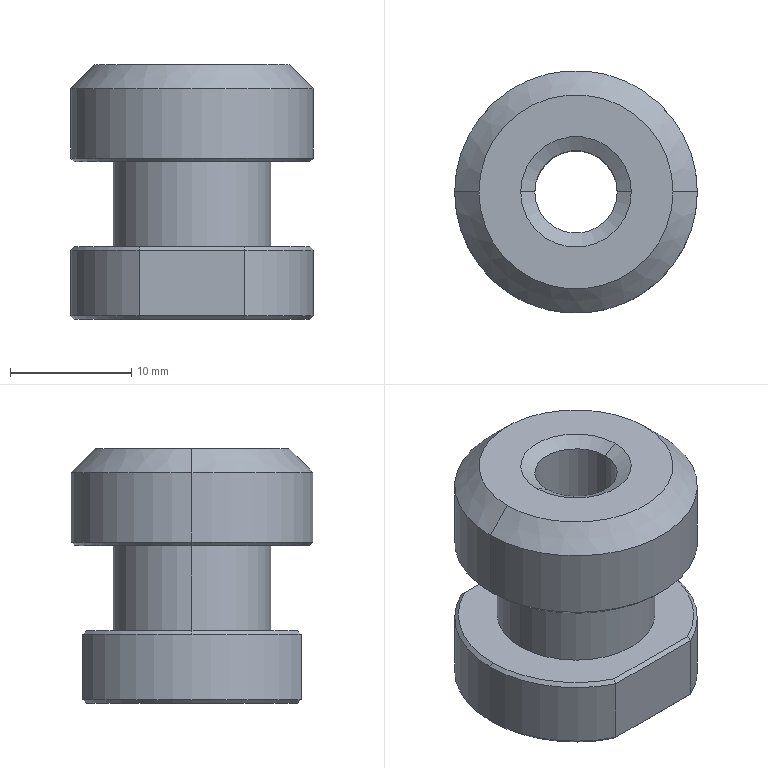Part | NX | 1 solid | 31 faces | box 20 x 20 x 21 mm | volume 4359 mm3 | cone 12 | plane 10 | cylinder 9 | commonest cylinder face diameters 20 x5 6.8 x2 13 x2
STEP:
#1=CARTESIAN_POINT('',(-93.533,-7.21,-2.7));
#2=VERTEX_POINT('',#1);
#3=CARTESIAN_POINT('',(-93.533,-7.21,2.7));
#4=VERTEX_POINT('',#3);
#5=CARTESIAN_POINT('',(-93.533,-7.21,-1.));
#6=DIRECTION('',(0.,0.,1.));
#7=VECTOR('',#6,1000.);
#8=LINE('',#5,#7);
#9=EDGE_CURVE('',#2,#4,#8,.T.);
#10=ORIENTED_EDGE('',*,*,#9,.F.);
#11=CARTESIAN_POINT('',(-99.174,1.79,-2.7));
#12=VERTEX_POINT('',#11);
#13=CARTESIAN_POINT('',(-103.533,-7.21,-2.7));
#14=DIRECTION('',(0.,0.,1.));
#15=DIRECTION('',(1.,0.,0.));
#16=AXIS2_PLACEMENT_3D('',#13,#14,#15);
#17=CIRCLE('',#16,10.);
#18=EDGE_CURVE('',#2,#12,#17,.T.);
#19=ORIENTED_EDGE('',*,*,#18,.T.);
#20=CARTESIAN_POINT('',(-99.174,1.79,2.7));
#21=VERTEX_POINT('',#20);
#22=CARTESIAN_POINT('',(-99.174,1.79,-1.));
#23=DIRECTION('',(0.,0.,1.));
#24=VECTOR('',#23,1000.);
#25=LINE('',#22,#24);
#26=EDGE_CURVE('',#12,#21,#25,.T.);
#27=ORIENTED_EDGE('',*,*,#26,.T.);
#28=CARTESIAN_POINT('',(-103.533,-7.21,2.7));
#29=DIRECTION('',(0.,0.,-1.));
#30=DIRECTION('',(-1.,0.,0.));
#31=AXIS2_PLACEMENT_3D('',#28,#29,#30);
#32=CIRCLE('',#31,10.);
#33=EDGE_CURVE('',#21,#4,#32,.T.);
#34=ORIENTED_EDGE('',*,*,#33,.T.);
#35=EDGE_LOOP('',(#10,#19,#27,#34));
#36=FACE_BOUND('',#35,.T.);
#37=CARTESIAN_POINT('',(-103.533,-7.21,-1.));
#38=DIRECTION('',(0.,0.,1.));
#39=DIRECTION('',(1.,0.,0.));
#40=AXIS2_PLACEMENT_3D('',#37,#38,#39);
#41=CYLINDRICAL_SURFACE('',#40,10.);
#42=ADVANCED_FACE('',(#36),#41,.T.);
#43=CARTESIAN_POINT('',(-107.892,1.79,-2.7));
#44=VERTEX_POINT('',#43);
#45=CARTESIAN_POINT('',(-107.892,1.79,2.7));
#46=VERTEX_POINT('',#45);
#47=CARTESIAN_POINT('',(-107.892,1.79,-1.));
#48=DIRECTION('',(0.,0.,1.));
#49=VECTOR('',#48,1000.);
#50=LINE('',#47,#49);
#51=EDGE_CURVE('',#44,#46,#50,.T.);
#52=ORIENTED_EDGE('',*,*,#51,.F.);
#53=CARTESIAN_POINT('',(-107.892,-16.21,-2.7));
#54=VERTEX_POINT('',#53);
#55=CARTESIAN_POINT('',(-103.533,-7.21,-2.7));
#56=DIRECTION('',(0.,0.,1.));
#57=DIRECTION('',(1.,0.,0.));
#58=AXIS2_PLACEMENT_3D('',#55,#56,#57);
#59=CIRCLE('',#58,10.);
#60=EDGE_CURVE('',#44,#54,#59,.T.);
#61=ORIENTED_EDGE('',*,*,#60,.T.);
#62=CARTESIAN_POINT('',(-107.892,-16.21,2.7));
#63=VERTEX_POINT('',#62);
#64=CARTESIAN_POINT('',(-107.892,-16.21,-1.));
#65=DIRECTION('',(0.,0.,1.));
#66=VECTOR('',#65,1000.);
#67=LINE('',#64,#66);
#68=EDGE_CURVE('',#54,#63,#67,.T.);
#69=ORIENTED_EDGE('',*,*,#68,.T.);
#70=CARTESIAN_POINT('',(-113.533,-7.21,2.7));
#71=VERTEX_POINT('',#70);
#72=CARTESIAN_POINT('',(-103.533,-7.21,2.7));
#73=DIRECTION('',(0.,0.,-1.));
#74=DIRECTION('',(-1.,0.,0.));
#75=AXIS2_PLACEMENT_3D('',#72,#73,#74);
#76=CIRCLE('',#75,10.);
#77=EDGE_CURVE('',#63,#71,#76,.T.);
#78=ORIENTED_EDGE('',*,*,#77,.T.);
#79=CARTESIAN_POINT('',(-103.533,-7.21,2.7));
#80=DIRECTION('',(0.,0.,-1.));
#81=DIRECTION('',(-1.,0.,0.));
#82=AXIS2_PLACEMENT_3D('',#79,#80,#81);
#83=CIRCLE('',#82,10.);
#84=EDGE_CURVE('',#71,#46,#83,.T.);
#85=ORIENTED_EDGE('',*,*,#84,.T.);
#86=EDGE_LOOP('',(#52,#61,#69,#78,#85));
#87=FACE_BOUND('',#86,.T.);
#88=CARTESIAN_POINT('',(-103.533,-7.21,-1.));
#89=DIRECTION('',(0.,0.,1.));
#90=DIRECTION('',(1.,0.,0.));
#91=AXIS2_PLACEMENT_3D('',#88,#89,#90);
#92=CYLINDRICAL_SURFACE('',#91,10.);
#93=ADVANCED_FACE('',(#87),#92,.T.);
#94=CARTESIAN_POINT('',(-99.174,-16.21,-2.7));
#95=VERTEX_POINT('',#94);
#96=CARTESIAN_POINT('',(-104.112,-16.21,-2.7));
#97=DIRECTION('',(-1.,0.,0.));
#98=VECTOR('',#97,1000.);
#99=LINE('',#96,#98);
#100=EDGE_CURVE('',#95,#54,#99,.T.);
#101=ORIENTED_EDGE('',*,*,#100,.F.);
#102=CARTESIAN_POINT('',(-99.174,-16.21,2.7));
#103=VERTEX_POINT('',#102);
#104=CARTESIAN_POINT('',(-99.174,-16.21,-1.));
#105=DIRECTION('',(0.,0.,1.));
#106=VECTOR('',#105,1000.);
#107=LINE('',#104,#106);
#108=EDGE_CURVE('',#95,#103,#107,.T.);
#109=ORIENTED_EDGE('',*,*,#108,.T.);
#110=CARTESIAN_POINT('',(-104.112,-16.21,2.7));
#111=DIRECTION('',(1.,0.,0.));
#112=VECTOR('',#111,1000.);
#113=LINE('',#110,#112);
#114=EDGE_CURVE('',#63,#103,#113,.T.);
#115=ORIENTED_EDGE('',*,*,#114,.F.);
#116=ORIENTED_EDGE('',*,*,#68,.F.);
#117=EDGE_LOOP('',(#101,#109,#115,#116));
#118=FACE_BOUND('',#117,.T.);
#119=CARTESIAN_POINT('',(-99.791,-16.21,-1.));
#120=DIRECTION('',(0.,-1.,0.));
#121=DIRECTION('',(0.,0.,-1.));
#122=AXIS2_PLACEMENT_3D('',#119,#120,#121);
#123=PLANE('',#122);
#124=ADVANCED_FACE('',(#118),#123,.T.);
#125=CARTESIAN_POINT('',(-99.243,-15.91,-3.));
#126=VERTEX_POINT('',#125);
#127=CARTESIAN_POINT('',(-107.822,-15.91,-3.));
#128=VERTEX_POINT('',#127);
#129=CARTESIAN_POINT('',(0.,-15.91,-3.));
#130=DIRECTION('',(-1.,0.,0.));
#131=VECTOR('',#130,1000.);
#132=LINE('',#129,#131);
#133=EDGE_CURVE('',#126,#128,#132,.T.);
#134=ORIENTED_EDGE('',*,*,#133,.F.);
#135=CARTESIAN_POINT('',(-99.174,-16.21,-2.7));
#136=CARTESIAN_POINT('',(-99.179,-16.185,-2.725));
#137=CARTESIAN_POINT('',(-99.185,-16.16,-2.75));
#138=CARTESIAN_POINT('',(-99.191,-16.135,-2.775));
#139=CARTESIAN_POINT('',(-99.197,-16.11,-2.8));
#140=CARTESIAN_POINT('',(-99.203,-16.085,-2.825));
#141=CARTESIAN_POINT('',(-99.208,-16.06,-2.85));
#142=CARTESIAN_POINT('',(-99.214,-16.035,-2.875));
#143=CARTESIAN_POINT('',(-99.22,-16.01,-2.9));
#144=CARTESIAN_POINT('',(-99.226,-15.985,-2.925));
#145=CARTESIAN_POINT('',(-99.231,-15.96,-2.95));
#146=CARTESIAN_POINT('',(-99.237,-15.935,-2.975));
#147=CARTESIAN_POINT('',(-99.243,-15.91,-3.));
#148=B_SPLINE_CURVE_WITH_KNOTS('',3,(#135,#136,#137,#138,#139,#140,#141,#142,#143,#144,#145,#146,#147),.UNSPECIFIED.,.F.,.F.,(4,3,3,3,4),(0.,0.1075,0.2149,0.3224,0.4299),.UNSPECIFIED.);
#149=EDGE_CURVE('',#95,#126,#148,.T.);
#150=ORIENTED_EDGE('',*,*,#149,.F.);
#151=ORIENTED_EDGE('',*,*,#100,.T.);
#152=CARTESIAN_POINT('',(-107.822,-15.91,-3.));
#153=CARTESIAN_POINT('',(-107.828,-15.935,-2.975));
#154=CARTESIAN_POINT('',(-107.834,-15.96,-2.95));
#155=CARTESIAN_POINT('',(-107.84,-15.985,-2.925));
#156=CARTESIAN_POINT('',(-107.845,-16.01,-2.9));
#157=CARTESIAN_POINT('',(-107.851,-16.035,-2.875));
#158=CARTESIAN_POINT('',(-107.857,-16.06,-2.85));
#159=CARTESIAN_POINT('',(-107.863,-16.085,-2.825));
#160=CARTESIAN_POINT('',(-107.869,-16.11,-2.8));
#161=CARTESIAN_POINT('',(-107.874,-16.135,-2.775));
#162=CARTESIAN_POINT('',(-107.88,-16.16,-2.75));
#163=CARTESIAN_POINT('',(-107.886,-16.185,-2.725));
#164=CARTESIAN_POINT('',(-107.892,-16.21,-2.7));
#165=B_SPLINE_CURVE_WITH_KNOTS('',3,(#152,#153,#154,#155,#156,#157,#158,#159,#160,#161,#162,#163,#164),.UNSPECIFIED.,.F.,.F.,(4,3,3,3,4),(0.,0.1075,0.2149,0.3224,0.4299),.UNSPECIFIED.);
#166=EDGE_CURVE('',#128,#54,#165,.T.);
#167=ORIENTED_EDGE('',*,*,#166,.F.);
#168=EDGE_LOOP('',(#134,#150,#151,#167));
#169=FACE_BOUND('',#168,.T.);
#170=CARTESIAN_POINT('',(-103.533,-16.06,-2.85));
#171=DIRECTION('',(0.,-0.7071,-0.7071));
#172=DIRECTION('',(0.,-0.7071,0.7071));
#173=AXIS2_PLACEMENT_3D('',#170,#171,#172);
#174=PLANE('',#173);
#175=ADVANCED_FACE('',(#169),#174,.T.);
#176=CARTESIAN_POINT('',(-107.822,1.49,-3.));
#177=VERTEX_POINT('',#176);
#178=CARTESIAN_POINT('',(-99.243,1.49,-3.));
#179=VERTEX_POINT('',#178);
#180=CARTESIAN_POINT('',(0.,1.49,-3.));
#181=DIRECTION('',(1.,0.,0.));
#182=VECTOR('',#181,1000.);
#183=LINE('',#180,#182);
#184=EDGE_CURVE('',#177,#179,#183,.T.);
#185=ORIENTED_EDGE('',*,*,#184,.F.);
#186=CARTESIAN_POINT('',(-107.892,1.79,-2.7));
#187=CARTESIAN_POINT('',(-107.886,1.765,-2.725));
#188=CARTESIAN_POINT('',(-107.88,1.74,-2.75));
#189=CARTESIAN_POINT('',(-107.874,1.715,-2.775));
#190=CARTESIAN_POINT('',(-107.869,1.69,-2.8));
#191=CARTESIAN_POINT('',(-107.863,1.665,-2.825));
#192=CARTESIAN_POINT('',(-107.857,1.64,-2.85));
#193=CARTESIAN_POINT('',(-107.851,1.615,-2.875));
#194=CARTESIAN_POINT('',(-107.845,1.59,-2.9));
#195=CARTESIAN_POINT('',(-107.84,1.565,-2.925));
#196=CARTESIAN_POINT('',(-107.834,1.54,-2.95));
#197=CARTESIAN_POINT('',(-107.828,1.515,-2.975));
#198=CARTESIAN_POINT('',(-107.822,1.49,-3.));
#199=B_SPLINE_CURVE_WITH_KNOTS('',3,(#186,#187,#188,#189,#190,#191,#192,#193,#194,#195,#196,#197,#198),.UNSPECIFIED.,.F.,.F.,(4,3,3,3,4),(0.,0.1075,0.2149,0.3224,0.4299),.UNSPECIFIED.);
#200=EDGE_CURVE('',#44,#177,#199,.T.);
#201=ORIENTED_EDGE('',*,*,#200,.F.);
#202=CARTESIAN_POINT('',(-104.112,1.79,-2.7));
#203=DIRECTION('',(1.,0.,0.));
#204=VECTOR('',#203,1000.);
#205=LINE('',#202,#204);
#206=EDGE_CURVE('',#44,#12,#205,.T.);
#207=ORIENTED_EDGE('',*,*,#206,.T.);
#208=CARTESIAN_POINT('',(-99.243,1.49,-3.));
#209=CARTESIAN_POINT('',(-99.237,1.515,-2.975));
#210=CARTESIAN_POINT('',(-99.231,1.54,-2.95));
#211=CARTESIAN_POINT('',(-99.226,1.565,-2.925));
#212=CARTESIAN_POINT('',(-99.22,1.59,-2.9));
#213=CARTESIAN_POINT('',(-99.214,1.615,-2.875));
#214=CARTESIAN_POINT('',(-99.208,1.64,-2.85));
#215=CARTESIAN_POINT('',(-99.203,1.665,-2.825));
#216=CARTESIAN_POINT('',(-99.197,1.69,-2.8));
#217=CARTESIAN_POINT('',(-99.191,1.715,-2.775));
#218=CARTESIAN_POINT('',(-99.185,1.74,-2.75));
#219=CARTESIAN_POINT('',(-99.179,1.765,-2.725));
#220=CARTESIAN_POINT('',(-99.174,1.79,-2.7));
#221=B_SPLINE_CURVE_WITH_KNOTS('',3,(#208,#209,#210,#211,#212,#213,#214,#215,#216,#217,#218,#219,#220),.UNSPECIFIED.,.F.,.F.,(4,3,3,3,4),(0.,0.1075,0.2149,0.3224,0.4299),.UNSPECIFIED.);
#222=EDGE_CURVE('',#179,#12,#221,.T.);
#223=ORIENTED_EDGE('',*,*,#222,.F.);
#224=EDGE_LOOP('',(#185,#201,#207,#223));
#225=FACE_BOUND('',#224,.T.);
#226=CARTESIAN_POINT('',(-103.533,1.64,-2.85));
#227=DIRECTION('',(0.,0.7071,-0.7071));
#228=DIRECTION('',(-1.,0.,0.));
#229=AXIS2_PLACEMENT_3D('',#226,#227,#228);
#230=PLANE('',#229);
#231=ADVANCED_FACE('',(#225),#230,.T.);
#232=CARTESIAN_POINT('',(-113.233,-7.21,10.));
#233=VERTEX_POINT('',#232);
#234=CARTESIAN_POINT('',(-93.833,-7.21,10.));
#235=VERTEX_POINT('',#234);
#236=CARTESIAN_POINT('',(-103.533,-7.21,10.));
#237=DIRECTION('',(0.,0.,1.));
#238=DIRECTION('',(1.,0.,0.));
#239=AXIS2_PLACEMENT_3D('',#236,#237,#238);
#240=CIRCLE('',#239,9.7);
#241=EDGE_CURVE('',#233,#235,#240,.T.);
#242=ORIENTED_EDGE('',*,*,#241,.F.);
#243=CARTESIAN_POINT('',(-103.533,-7.21,10.));
#244=DIRECTION('',(0.,0.,1.));
#245=DIRECTION('',(1.,0.,0.));
#246=AXIS2_PLACEMENT_3D('',#243,#244,#245);
#247=CIRCLE('',#246,9.7);
#248=EDGE_CURVE('',#235,#233,#247,.T.);
#249=ORIENTED_EDGE('',*,*,#248,.F.);
#250=EDGE_LOOP('',(#242,#249));
#251=FACE_BOUND('',#250,.T.);
#252=CARTESIAN_POINT('',(-97.033,-7.21,10.));
#253=VERTEX_POINT('',#252);
#254=CARTESIAN_POINT('',(-110.033,-7.21,10.));
#255=VERTEX_POINT('',#254);
#256=CARTESIAN_POINT('',(-103.533,-7.21,10.));
#257=DIRECTION('',(0.,0.,1.));
#258=DIRECTION('',(1.,0.,0.));
#259=AXIS2_PLACEMENT_3D('',#256,#257,#258);
#260=CIRCLE('',#259,6.5);
#261=EDGE_CURVE('',#253,#255,#260,.T.);
#262=ORIENTED_EDGE('',*,*,#261,.T.);
#263=CARTESIAN_POINT('',(-103.533,-7.21,10.));
#264=DIRECTION('',(0.,0.,1.));
#265=DIRECTION('',(1.,0.,0.));
#266=AXIS2_PLACEMENT_3D('',#263,#264,#265);
#267=CIRCLE('',#266,6.5);
#268=EDGE_CURVE('',#255,#253,#267,.T.);
#269=ORIENTED_EDGE('',*,*,#268,.T.);
#270=EDGE_LOOP('',(#262,#269));
#271=FACE_BOUND('',#270,.T.);
#272=CARTESIAN_POINT('',(-103.03,-7.592,10.));
#273=DIRECTION('',(0.,0.,1.));
#274=DIRECTION('',(1.,0.,0.));
#275=AXIS2_PLACEMENT_3D('',#272,#273,#274);
#276=PLANE('',#275);
#277=ADVANCED_FACE('',(#251,#271),#276,.F.);
#278=CARTESIAN_POINT('',(-110.033,-7.21,3.));
#279=VERTEX_POINT('',#278);
#280=CARTESIAN_POINT('',(-97.033,-7.21,3.));
#281=VERTEX_POINT('',#280);
#282=CARTESIAN_POINT('',(-103.533,-7.21,3.));
#283=DIRECTION('',(0.,0.,1.));
#284=DIRECTION('',(1.,0.,0.));
#285=AXIS2_PLACEMENT_3D('',#282,#283,#284);
#286=CIRCLE('',#285,6.5);
#287=EDGE_CURVE('',#279,#281,#286,.T.);
#288=ORIENTED_EDGE('',*,*,#287,.T.);
#289=CARTESIAN_POINT('',(-97.033,-7.21,5.));
#290=DIRECTION('',(0.,0.,1.));
#291=VECTOR('',#290,1000.);
#292=LINE('',#289,#291);
#293=EDGE_CURVE('',#281,#253,#292,.T.);
#294=ORIENTED_EDGE('',*,*,#293,.T.);
#295=ORIENTED_EDGE('',*,*,#268,.F.);
#296=CARTESIAN_POINT('',(-110.033,-7.21,5.));
#297=DIRECTION('',(0.,0.,1.));
#298=VECTOR('',#297,1000.);
#299=LINE('',#296,#298);
#300=EDGE_CURVE('',#279,#255,#299,.T.);
#301=ORIENTED_EDGE('',*,*,#300,.F.);
#302=EDGE_LOOP('',(#288,#294,#295,#301));
#303=FACE_BOUND('',#302,.T.);
#304=CARTESIAN_POINT('',(-103.533,-7.21,5.));
#305=DIRECTION('',(0.,0.,1.));
#306=DIRECTION('',(1.,0.,0.));
#307=AXIS2_PLACEMENT_3D('',#304,#305,#306);
#308=CYLINDRICAL_SURFACE('',#307,6.5);
#309=ADVANCED_FACE('',(#303),#308,.T.);
#310=CARTESIAN_POINT('',(-107.822,1.49,3.));
#311=VERTEX_POINT('',#310);
#312=CARTESIAN_POINT('',(-99.243,1.49,3.));
#313=VERTEX_POINT('',#312);
#314=CARTESIAN_POINT('',(-104.112,1.49,3.));
#315=DIRECTION('',(1.,0.,0.));
#316=VECTOR('',#315,1000.);
#317=LINE('',#314,#316);
#318=EDGE_CURVE('',#311,#313,#317,.T.);
#319=ORIENTED_EDGE('',*,*,#318,.F.);
#320=CARTESIAN_POINT('',(-113.233,-7.21,3.));
#321=VERTEX_POINT('',#320);
#322=CARTESIAN_POINT('',(-103.533,-7.21,3.));
#323=DIRECTION('',(0.,0.,-1.));
#324=DIRECTION('',(-1.,0.,0.));
#325=AXIS2_PLACEMENT_3D('',#322,#323,#324);
#326=CIRCLE('',#325,9.7);
#327=EDGE_CURVE('',#321,#311,#326,.T.);
#328=ORIENTED_EDGE('',*,*,#327,.F.);
#329=CARTESIAN_POINT('',(-107.822,-15.91,3.));
#330=VERTEX_POINT('',#329);
#331=CARTESIAN_POINT('',(-103.533,-7.21,3.));
#332=DIRECTION('',(0.,0.,-1.));
#333=DIRECTION('',(-1.,0.,0.));
#334=AXIS2_PLACEMENT_3D('',#331,#332,#333);
#335=CIRCLE('',#334,9.7);
#336=EDGE_CURVE('',#330,#321,#335,.T.);
#337=ORIENTED_EDGE('',*,*,#336,.F.);
#338=CARTESIAN_POINT('',(-99.243,-15.91,3.));
#339=VERTEX_POINT('',#338);
#340=CARTESIAN_POINT('',(-104.112,-15.91,3.));
#341=DIRECTION('',(-1.,0.,0.));
#342=VECTOR('',#341,1000.);
#343=LINE('',#340,#342);
#344=EDGE_CURVE('',#339,#330,#343,.T.);
#345=ORIENTED_EDGE('',*,*,#344,.F.);
#346=CARTESIAN_POINT('',(-103.533,-7.21,3.));
#347=DIRECTION('',(0.,0.,-1.));
#348=DIRECTION('',(-1.,0.,0.));
#349=AXIS2_PLACEMENT_3D('',#346,#347,#348);
#350=CIRCLE('',#349,9.7);
#351=EDGE_CURVE('',#313,#339,#350,.T.);
#352=ORIENTED_EDGE('',*,*,#351,.F.);
#353=EDGE_LOOP('',(#319,#328,#337,#345,#352));
#354=FACE_BOUND('',#353,.T.);
#355=ORIENTED_EDGE('',*,*,#287,.F.);
#356=CARTESIAN_POINT('',(-103.533,-7.21,3.));
#357=DIRECTION('',(0.,0.,1.));
#358=DIRECTION('',(1.,0.,0.));
#359=AXIS2_PLACEMENT_3D('',#356,#357,#358);
#360=CIRCLE('',#359,6.5);
#361=EDGE_CURVE('',#281,#279,#360,.T.);
#362=ORIENTED_EDGE('',*,*,#361,.F.);
#363=EDGE_LOOP('',(#355,#362));
#364=FACE_BOUND('',#363,.T.);
#365=CARTESIAN_POINT('',(-104.112,-7.022,3.));
#366=DIRECTION('',(0.,0.,1.));
#367=DIRECTION('',(1.,0.,0.));
#368=AXIS2_PLACEMENT_3D('',#365,#366,#367);
#369=PLANE('',#368);
#370=ADVANCED_FACE('',(#354,#364),#369,.T.);
#371=CARTESIAN_POINT('',(-113.533,-7.21,16.));
#372=VERTEX_POINT('',#371);
#373=CARTESIAN_POINT('',(-93.533,-7.21,16.));
#374=VERTEX_POINT('',#373);
#375=CARTESIAN_POINT('',(-103.533,-7.21,16.));
#376=DIRECTION('',(0.,0.,-1.));
#377=DIRECTION('',(-1.,0.,0.));
#378=AXIS2_PLACEMENT_3D('',#375,#376,#377);
#379=CIRCLE('',#378,10.);
#380=EDGE_CURVE('',#372,#374,#379,.T.);
#381=ORIENTED_EDGE('',*,*,#380,.T.);
#382=CARTESIAN_POINT('',(-93.533,-7.21,10.3));
#383=VERTEX_POINT('',#382);
#384=CARTESIAN_POINT('',(-93.533,-7.21,10.));
#385=DIRECTION('',(0.,0.,1.));
#386=VECTOR('',#385,1000.);
#387=LINE('',#384,#386);
#388=EDGE_CURVE('',#383,#374,#387,.T.);
#389=ORIENTED_EDGE('',*,*,#388,.F.);
#390=CARTESIAN_POINT('',(-113.533,-7.21,10.3));
#391=VERTEX_POINT('',#390);
#392=CARTESIAN_POINT('',(-103.533,-7.21,10.3));
#393=DIRECTION('',(0.,0.,1.));
#394=DIRECTION('',(1.,0.,0.));
#395=AXIS2_PLACEMENT_3D('',#392,#393,#394);
#396=CIRCLE('',#395,10.);
#397=EDGE_CURVE('',#383,#391,#396,.T.);
#398=ORIENTED_EDGE('',*,*,#397,.T.);
#399=CARTESIAN_POINT('',(-113.533,-7.21,10.));
#400=DIRECTION('',(0.,0.,1.));
#401=VECTOR('',#400,1000.);
#402=LINE('',#399,#401);
#403=EDGE_CURVE('',#391,#372,#402,.T.);
#404=ORIENTED_EDGE('',*,*,#403,.T.);
#405=EDGE_LOOP('',(#381,#389,#398,#404));
#406=FACE_BOUND('',#405,.T.);
#407=CARTESIAN_POINT('',(-103.533,-7.21,10.));
#408=DIRECTION('',(0.,0.,1.));
#409=DIRECTION('',(1.,0.,0.));
#410=AXIS2_PLACEMENT_3D('',#407,#408,#409);
#411=CYLINDRICAL_SURFACE('',#410,10.);
#412=ADVANCED_FACE('',(#406),#411,.T.);
#413=CARTESIAN_POINT('',(-95.533,-7.21,18.));
#414=VERTEX_POINT('',#413);
#415=CARTESIAN_POINT('',(-111.533,-7.21,18.));
#416=VERTEX_POINT('',#415);
#417=CARTESIAN_POINT('',(-103.533,-7.21,18.));
#418=DIRECTION('',(0.,0.,-1.));
#419=DIRECTION('',(-1.,0.,0.));
#420=AXIS2_PLACEMENT_3D('',#417,#418,#419);
#421=CIRCLE('',#420,8.);
#422=EDGE_CURVE('',#414,#416,#421,.T.);
#423=ORIENTED_EDGE('',*,*,#422,.F.);
#424=CARTESIAN_POINT('',(-103.533,-7.21,18.));
#425=DIRECTION('',(0.,0.,-1.));
#426=DIRECTION('',(-1.,0.,0.));
#427=AXIS2_PLACEMENT_3D('',#424,#425,#426);
#428=CIRCLE('',#427,8.);
#429=EDGE_CURVE('',#416,#414,#428,.T.);
#430=ORIENTED_EDGE('',*,*,#429,.F.);
#431=EDGE_LOOP('',(#423,#430));
#432=FACE_BOUND('',#431,.T.);
#433=CARTESIAN_POINT('',(-98.97,-7.21,18.));
#434=VERTEX_POINT('',#433);
#435=CARTESIAN_POINT('',(-108.095,-7.21,18.));
#436=VERTEX_POINT('',#435);
#437=CARTESIAN_POINT('',(-103.533,-7.21,18.));
#438=DIRECTION('',(0.,0.,1.));
#439=DIRECTION('',(1.,0.,0.));
#440=AXIS2_PLACEMENT_3D('',#437,#438,#439);
#441=CIRCLE('',#440,4.562);
#442=EDGE_CURVE('',#434,#436,#441,.T.);
#443=ORIENTED_EDGE('',*,*,#442,.F.);
#444=CARTESIAN_POINT('',(-103.533,-7.21,18.));
#445=DIRECTION('',(0.,0.,1.));
#446=DIRECTION('',(1.,0.,0.));
#447=AXIS2_PLACEMENT_3D('',#444,#445,#446);
#448=CIRCLE('',#447,4.562);
#449=EDGE_CURVE('',#436,#434,#448,.T.);
#450=ORIENTED_EDGE('',*,*,#449,.F.);
#451=EDGE_LOOP('',(#443,#450));
#452=FACE_BOUND('',#451,.T.);
#453=CARTESIAN_POINT('',(-103.03,-7.592,18.));
#454=DIRECTION('',(0.,0.,1.));
#455=DIRECTION('',(1.,0.,0.));
#456=AXIS2_PLACEMENT_3D('',#453,#454,#455);
#457=PLANE('',#456);
#458=ADVANCED_FACE('',(#432,#452),#457,.T.);
#459=ORIENTED_EDGE('',*,*,#206,.F.);
#460=ORIENTED_EDGE('',*,*,#51,.T.);
#461=CARTESIAN_POINT('',(-104.112,1.79,2.7));
#462=DIRECTION('',(-1.,0.,0.));
#463=VECTOR('',#462,1000.);
#464=LINE('',#461,#463);
#465=EDGE_CURVE('',#21,#46,#464,.T.);
#466=ORIENTED_EDGE('',*,*,#465,.F.);
#467=ORIENTED_EDGE('',*,*,#26,.F.);
#468=EDGE_LOOP('',(#459,#460,#466,#467));
#469=FACE_BOUND('',#468,.T.);
#470=CARTESIAN_POINT('',(-107.274,1.79,-1.));
#471=DIRECTION('',(0.,1.,0.));
#472=DIRECTION('',(1.,0.,0.));
#473=AXIS2_PLACEMENT_3D('',#470,#471,#472);
#474=PLANE('',#473);
#475=ADVANCED_FACE('',(#469),#474,.T.);
#476=CARTESIAN_POINT('',(-93.833,-7.21,-3.));
#477=VERTEX_POINT('',#476);
#478=CARTESIAN_POINT('',(-93.833,-7.21,-3.));
#479=DIRECTION('',(0.7071,0.,0.7071));
#480=VECTOR('',#479,1000.);
#481=LINE('',#478,#480);
#482=EDGE_CURVE('',#477,#2,#481,.T.);
#483=ORIENTED_EDGE('',*,*,#482,.F.);
#484=CARTESIAN_POINT('',(-103.533,-7.21,-3.));
#485=DIRECTION('',(0.,0.,1.));
#486=DIRECTION('',(1.,0.,0.));
#487=AXIS2_PLACEMENT_3D('',#484,#485,#486);
#488=CIRCLE('',#487,9.7);
#489=EDGE_CURVE('',#477,#179,#488,.T.);
#490=ORIENTED_EDGE('',*,*,#489,.T.);
#491=ORIENTED_EDGE('',*,*,#222,.T.);
#492=ORIENTED_EDGE('',*,*,#18,.F.);
#493=EDGE_LOOP('',(#483,#490,#491,#492));
#494=FACE_BOUND('',#493,.T.);
#495=CARTESIAN_POINT('',(-103.533,-7.21,-3.));
#496=DIRECTION('',(0.,0.,1.));
#497=DIRECTION('',(1.,0.,0.));
#498=AXIS2_PLACEMENT_3D('',#495,#496,#497);
#499=CONICAL_SURFACE('',#498,9.7,0.7854);
#500=ADVANCED_FACE('',(#494),#499,.T.);
#501=ORIENTED_EDGE('',*,*,#380,.F.);
#502=CARTESIAN_POINT('',(-111.533,-7.21,18.));
#503=DIRECTION('',(-0.7071,0.,-0.7071));
#504=VECTOR('',#503,1000.);
#505=LINE('',#502,#504);
#506=EDGE_CURVE('',#372,#416,#505,.F.);
#507=ORIENTED_EDGE('',*,*,#506,.T.);
#508=ORIENTED_EDGE('',*,*,#429,.T.);
#509=CARTESIAN_POINT('',(-95.533,-7.21,18.));
#510=DIRECTION('',(0.7071,0.,-0.7071));
#511=VECTOR('',#510,1000.);
#512=LINE('',#509,#511);
#513=EDGE_CURVE('',#374,#414,#512,.F.);
#514=ORIENTED_EDGE('',*,*,#513,.F.);
#515=EDGE_LOOP('',(#501,#507,#508,#514));
#516=FACE_BOUND('',#515,.T.);
#517=CARTESIAN_POINT('',(-103.533,-7.21,18.));
#518=DIRECTION('',(0.,0.,-1.));
#519=DIRECTION('',(-1.,0.,0.));
#520=AXIS2_PLACEMENT_3D('',#517,#518,#519);
#521=CONICAL_SURFACE('',#520,8.,0.7854);
#522=ADVANCED_FACE('',(#516),#521,.T.);
#523=CARTESIAN_POINT('',(-103.533,-7.21,-3.));
#524=DIRECTION('',(0.,0.,1.));
#525=DIRECTION('',(1.,0.,0.));
#526=AXIS2_PLACEMENT_3D('',#523,#524,#525);
#527=CIRCLE('',#526,9.7);
#528=EDGE_CURVE('',#177,#128,#527,.T.);
#529=ORIENTED_EDGE('',*,*,#528,.T.);
#530=ORIENTED_EDGE('',*,*,#166,.T.);
#531=ORIENTED_EDGE('',*,*,#60,.F.);
#532=ORIENTED_EDGE('',*,*,#200,.T.);
#533=EDGE_LOOP('',(#529,#530,#531,#532));
#534=FACE_BOUND('',#533,.T.);
#535=CARTESIAN_POINT('',(-103.533,-7.21,-3.));
#536=DIRECTION('',(0.,0.,1.));
#537=DIRECTION('',(1.,0.,0.));
#538=AXIS2_PLACEMENT_3D('',#535,#536,#537);
#539=CONICAL_SURFACE('',#538,9.7,0.7854);
#540=ADVANCED_FACE('',(#534),#539,.T.);
#541=ORIENTED_EDGE('',*,*,#241,.T.);
#542=CARTESIAN_POINT('',(-93.833,-7.21,10.));
#543=DIRECTION('',(0.7071,0.,0.7071));
#544=VECTOR('',#543,1000.);
#545=LINE('',#542,#544);
#546=EDGE_CURVE('',#235,#383,#545,.T.);
#547=ORIENTED_EDGE('',*,*,#546,.T.);
#548=CARTESIAN_POINT('',(-103.533,-7.21,10.3));
#549=DIRECTION('',(0.,0.,1.));
#550=DIRECTION('',(1.,0.,0.));
#551=AXIS2_PLACEMENT_3D('',#548,#549,#550);
#552=CIRCLE('',#551,10.);
#553=EDGE_CURVE('',#391,#383,#552,.T.);
#554=ORIENTED_EDGE('',*,*,#553,.F.);
#555=CARTESIAN_POINT('',(-113.233,-7.21,10.));
#556=DIRECTION('',(-0.7071,0.,0.7071));
#557=VECTOR('',#556,1000.);
#558=LINE('',#555,#557);
#559=EDGE_CURVE('',#233,#391,#558,.T.);
#560=ORIENTED_EDGE('',*,*,#559,.F.);
#561=EDGE_LOOP('',(#541,#547,#554,#560));
#562=FACE_BOUND('',#561,.T.);
#563=CARTESIAN_POINT('',(-103.533,-7.21,10.));
#564=DIRECTION('',(0.,0.,1.));
#565=DIRECTION('',(1.,0.,0.));
#566=AXIS2_PLACEMENT_3D('',#563,#564,#565);
#567=CONICAL_SURFACE('',#566,9.7,0.7854);
#568=ADVANCED_FACE('',(#562),#567,.T.);
#569=ORIENTED_EDGE('',*,*,#351,.T.);
#570=CARTESIAN_POINT('',(-99.174,-16.21,2.7));
#571=CARTESIAN_POINT('',(-99.179,-16.185,2.725));
#572=CARTESIAN_POINT('',(-99.185,-16.16,2.75));
#573=CARTESIAN_POINT('',(-99.191,-16.135,2.775));
#574=CARTESIAN_POINT('',(-99.197,-16.11,2.8));
#575=CARTESIAN_POINT('',(-99.203,-16.085,2.825));
#576=CARTESIAN_POINT('',(-99.208,-16.06,2.85));
#577=CARTESIAN_POINT('',(-99.214,-16.035,2.875));
#578=CARTESIAN_POINT('',(-99.22,-16.01,2.9));
#579=CARTESIAN_POINT('',(-99.226,-15.985,2.925));
#580=CARTESIAN_POINT('',(-99.231,-15.96,2.95));
#581=CARTESIAN_POINT('',(-99.237,-15.935,2.975));
#582=CARTESIAN_POINT('',(-99.243,-15.91,3.));
#583=B_SPLINE_CURVE_WITH_KNOTS('',3,(#570,#571,#572,#573,#574,#575,#576,#577,#578,#579,#580,#581,#582),.UNSPECIFIED.,.F.,.F.,(4,3,3,3,4),(0.,0.1075,0.2149,0.3224,0.4299),.UNSPECIFIED.);
#584=EDGE_CURVE('',#103,#339,#583,.T.);
#585=ORIENTED_EDGE('',*,*,#584,.F.);
#586=CARTESIAN_POINT('',(-103.533,-7.21,2.7));
#587=DIRECTION('',(0.,0.,-1.));
#588=DIRECTION('',(-1.,0.,0.));
#589=AXIS2_PLACEMENT_3D('',#586,#587,#588);
#590=CIRCLE('',#589,10.);
#591=EDGE_CURVE('',#4,#103,#590,.T.);
#592=ORIENTED_EDGE('',*,*,#591,.F.);
#593=ORIENTED_EDGE('',*,*,#33,.F.);
#594=CARTESIAN_POINT('',(-99.243,1.49,3.));
#595=CARTESIAN_POINT('',(-99.237,1.515,2.975));
#596=CARTESIAN_POINT('',(-99.231,1.54,2.95));
#597=CARTESIAN_POINT('',(-99.226,1.565,2.925));
#598=CARTESIAN_POINT('',(-99.22,1.59,2.9));
#599=CARTESIAN_POINT('',(-99.214,1.615,2.875));
#600=CARTESIAN_POINT('',(-99.208,1.64,2.85));
#601=CARTESIAN_POINT('',(-99.203,1.665,2.825));
#602=CARTESIAN_POINT('',(-99.197,1.69,2.8));
#603=CARTESIAN_POINT('',(-99.191,1.715,2.775));
#604=CARTESIAN_POINT('',(-99.185,1.74,2.75));
#605=CARTESIAN_POINT('',(-99.179,1.765,2.725));
#606=CARTESIAN_POINT('',(-99.174,1.79,2.7));
#607=B_SPLINE_CURVE_WITH_KNOTS('',3,(#594,#595,#596,#597,#598,#599,#600,#601,#602,#603,#604,#605,#606),.UNSPECIFIED.,.F.,.F.,(4,3,3,3,4),(0.,0.1075,0.2149,0.3224,0.4299),.UNSPECIFIED.);
#608=EDGE_CURVE('',#313,#21,#607,.T.);
#609=ORIENTED_EDGE('',*,*,#608,.F.);
#610=EDGE_LOOP('',(#569,#585,#592,#593,#609));
#611=FACE_BOUND('',#610,.T.);
#612=CARTESIAN_POINT('',(-103.533,-7.21,3.));
#613=DIRECTION('',(0.,0.,-1.));
#614=DIRECTION('',(-1.,0.,0.));
#615=AXIS2_PLACEMENT_3D('',#612,#613,#614);
#616=CONICAL_SURFACE('',#615,9.7,0.7854);
#617=ADVANCED_FACE('',(#611),#616,.T.);
#618=ORIENTED_EDGE('',*,*,#344,.T.);
#619=CARTESIAN_POINT('',(-107.822,-15.91,3.));
#620=CARTESIAN_POINT('',(-107.828,-15.935,2.975));
#621=CARTESIAN_POINT('',(-107.834,-15.96,2.95));
#622=CARTESIAN_POINT('',(-107.84,-15.985,2.925));
#623=CARTESIAN_POINT('',(-107.845,-16.01,2.9));
#624=CARTESIAN_POINT('',(-107.851,-16.035,2.875));
#625=CARTESIAN_POINT('',(-107.857,-16.06,2.85));
#626=CARTESIAN_POINT('',(-107.863,-16.085,2.825));
#627=CARTESIAN_POINT('',(-107.869,-16.11,2.8));
#628=CARTESIAN_POINT('',(-107.874,-16.135,2.775));
#629=CARTESIAN_POINT('',(-107.88,-16.16,2.75));
#630=CARTESIAN_POINT('',(-107.886,-16.185,2.725));
#631=CARTESIAN_POINT('',(-107.892,-16.21,2.7));
#632=B_SPLINE_CURVE_WITH_KNOTS('',3,(#619,#620,#621,#622,#623,#624,#625,#626,#627,#628,#629,#630,#631),.UNSPECIFIED.,.F.,.F.,(4,3,3,3,4),(0.,0.1075,0.2149,0.3224,0.4299),.UNSPECIFIED.);
#633=EDGE_CURVE('',#330,#63,#632,.T.);
#634=ORIENTED_EDGE('',*,*,#633,.T.);
#635=ORIENTED_EDGE('',*,*,#114,.T.);
#636=ORIENTED_EDGE('',*,*,#584,.T.);
#637=EDGE_LOOP('',(#618,#634,#635,#636));
#638=FACE_BOUND('',#637,.T.);
#639=CARTESIAN_POINT('',(-103.533,-16.06,2.85));
#640=DIRECTION('',(0.,-0.7071,0.7071));
#641=DIRECTION('',(-1.,0.,0.));
#642=AXIS2_PLACEMENT_3D('',#639,#640,#641);
#643=PLANE('',#642);
#644=ADVANCED_FACE('',(#638),#643,.T.);
#645=CARTESIAN_POINT('',(-113.233,-7.21,3.));
#646=DIRECTION('',(-0.7071,0.,-0.7071));
#647=VECTOR('',#646,1000.);
#648=LINE('',#645,#647);
#649=EDGE_CURVE('',#321,#71,#648,.T.);
#650=ORIENTED_EDGE('',*,*,#649,.F.);
#651=ORIENTED_EDGE('',*,*,#327,.T.);
#652=CARTESIAN_POINT('',(-107.822,1.49,3.));
#653=CARTESIAN_POINT('',(-107.828,1.515,2.975));
#654=CARTESIAN_POINT('',(-107.834,1.54,2.95));
#655=CARTESIAN_POINT('',(-107.84,1.565,2.925));
#656=CARTESIAN_POINT('',(-107.845,1.59,2.9));
#657=CARTESIAN_POINT('',(-107.851,1.615,2.875));
#658=CARTESIAN_POINT('',(-107.857,1.64,2.85));
#659=CARTESIAN_POINT('',(-107.863,1.665,2.825));
#660=CARTESIAN_POINT('',(-107.869,1.69,2.8));
#661=CARTESIAN_POINT('',(-107.874,1.715,2.775));
#662=CARTESIAN_POINT('',(-107.88,1.74,2.75));
#663=CARTESIAN_POINT('',(-107.886,1.765,2.725));
#664=CARTESIAN_POINT('',(-107.892,1.79,2.7));
#665=B_SPLINE_CURVE_WITH_KNOTS('',3,(#652,#653,#654,#655,#656,#657,#658,#659,#660,#661,#662,#663,#664),.UNSPECIFIED.,.F.,.F.,(4,3,3,3,4),(0.,0.1075,0.2149,0.3224,0.4299),.UNSPECIFIED.);
#666=EDGE_CURVE('',#311,#46,#665,.T.);
#667=ORIENTED_EDGE('',*,*,#666,.T.);
#668=ORIENTED_EDGE('',*,*,#84,.F.);
#669=EDGE_LOOP('',(#650,#651,#667,#668));
#670=FACE_BOUND('',#669,.T.);
#671=CARTESIAN_POINT('',(-103.533,-7.21,3.));
#672=DIRECTION('',(0.,0.,-1.));
#673=DIRECTION('',(-1.,0.,0.));
#674=AXIS2_PLACEMENT_3D('',#671,#672,#673);
#675=CONICAL_SURFACE('',#674,9.7,0.7854);
#676=ADVANCED_FACE('',(#670),#675,.T.);
#677=ORIENTED_EDGE('',*,*,#318,.T.);
#678=ORIENTED_EDGE('',*,*,#608,.T.);
#679=ORIENTED_EDGE('',*,*,#465,.T.);
#680=ORIENTED_EDGE('',*,*,#666,.F.);
#681=EDGE_LOOP('',(#677,#678,#679,#680));
#682=FACE_BOUND('',#681,.T.);
#683=CARTESIAN_POINT('',(-103.533,1.64,2.85));
#684=DIRECTION('',(0.,0.7071,0.7071));
#685=DIRECTION('',(1.,0.,0.));
#686=AXIS2_PLACEMENT_3D('',#683,#684,#685);
#687=PLANE('',#686);
#688=ADVANCED_FACE('',(#682),#687,.T.);
#689=ORIENTED_EDGE('',*,*,#184,.T.);
#690=ORIENTED_EDGE('',*,*,#489,.F.);
#691=CARTESIAN_POINT('',(-103.533,-7.21,-3.));
#692=DIRECTION('',(0.,0.,1.));
#693=DIRECTION('',(1.,0.,0.));
#694=AXIS2_PLACEMENT_3D('',#691,#692,#693);
#695=CIRCLE('',#694,9.7);
#696=EDGE_CURVE('',#126,#477,#695,.T.);
#697=ORIENTED_EDGE('',*,*,#696,.F.);
#698=ORIENTED_EDGE('',*,*,#133,.T.);
#699=ORIENTED_EDGE('',*,*,#528,.F.);
#700=EDGE_LOOP('',(#689,#690,#697,#698,#699));
#701=FACE_BOUND('',#700,.T.);
#702=CARTESIAN_POINT('',(-100.133,-7.21,-3.));
#703=VERTEX_POINT('',#702);
#704=CARTESIAN_POINT('',(-106.933,-7.21,-3.));
#705=VERTEX_POINT('',#704);
#706=CARTESIAN_POINT('',(-103.533,-7.21,-3.));
#707=DIRECTION('',(0.,0.,1.));
#708=DIRECTION('',(1.,0.,0.));
#709=AXIS2_PLACEMENT_3D('',#706,#707,#708);
#710=CIRCLE('',#709,3.4);
#711=EDGE_CURVE('',#703,#705,#710,.T.);
#712=ORIENTED_EDGE('',*,*,#711,.T.);
#713=CARTESIAN_POINT('',(-103.533,-7.21,-3.));
#714=DIRECTION('',(0.,0.,1.));
#715=DIRECTION('',(1.,0.,0.));
#716=AXIS2_PLACEMENT_3D('',#713,#714,#715);
#717=CIRCLE('',#716,3.4);
#718=EDGE_CURVE('',#705,#703,#717,.T.);
#719=ORIENTED_EDGE('',*,*,#718,.T.);
#720=EDGE_LOOP('',(#712,#719));
#721=FACE_BOUND('',#720,.T.);
#722=CARTESIAN_POINT('',(-104.112,-7.022,-3.));
#723=DIRECTION('',(0.,0.,1.));
#724=DIRECTION('',(1.,0.,0.));
#725=AXIS2_PLACEMENT_3D('',#722,#723,#724);
#726=PLANE('',#725);
#727=ADVANCED_FACE('',(#701,#721),#726,.F.);
#728=CARTESIAN_POINT('',(-100.133,-7.21,17.329));
#729=VERTEX_POINT('',#728);
#730=CARTESIAN_POINT('',(-106.933,-7.21,17.329));
#731=VERTEX_POINT('',#730);
#732=CARTESIAN_POINT('',(-103.533,-7.21,17.329));
#733=DIRECTION('',(0.,0.,1.));
#734=DIRECTION('',(1.,0.,0.));
#735=AXIS2_PLACEMENT_3D('',#732,#733,#734);
#736=CIRCLE('',#735,3.4);
#737=EDGE_CURVE('',#729,#731,#736,.T.);
#738=ORIENTED_EDGE('',*,*,#737,.T.);
#739=CARTESIAN_POINT('',(-106.933,-7.21,18.));
#740=DIRECTION('',(0.,0.,1.));
#741=VECTOR('',#740,1000.);
#742=LINE('',#739,#741);
#743=EDGE_CURVE('',#705,#731,#742,.T.);
#744=ORIENTED_EDGE('',*,*,#743,.F.);
#745=ORIENTED_EDGE('',*,*,#711,.F.);
#746=CARTESIAN_POINT('',(-100.133,-7.21,18.));
#747=DIRECTION('',(0.,0.,1.));
#748=VECTOR('',#747,1000.);
#749=LINE('',#746,#748);
#750=EDGE_CURVE('',#703,#729,#749,.T.);
#751=ORIENTED_EDGE('',*,*,#750,.T.);
#752=EDGE_LOOP('',(#738,#744,#745,#751));
#753=FACE_BOUND('',#752,.T.);
#754=CARTESIAN_POINT('',(-103.533,-7.21,18.));
#755=DIRECTION('',(0.,0.,1.));
#756=DIRECTION('',(1.,0.,0.));
#757=AXIS2_PLACEMENT_3D('',#754,#755,#756);
#758=CYLINDRICAL_SURFACE('',#757,3.4);
#759=ADVANCED_FACE('',(#753),#758,.F.);
#760=ORIENTED_EDGE('',*,*,#737,.F.);
#761=CARTESIAN_POINT('',(-100.133,-7.21,17.329));
#762=DIRECTION('',(0.866,0.,0.5));
#763=VECTOR('',#762,1000.);
#764=LINE('',#761,#763);
#765=EDGE_CURVE('',#729,#434,#764,.T.);
#766=ORIENTED_EDGE('',*,*,#765,.T.);
#767=ORIENTED_EDGE('',*,*,#442,.T.);
#768=CARTESIAN_POINT('',(-106.933,-7.21,17.329));
#769=DIRECTION('',(-0.866,0.,0.5));
#770=VECTOR('',#769,1000.);
#771=LINE('',#768,#770);
#772=EDGE_CURVE('',#731,#436,#771,.T.);
#773=ORIENTED_EDGE('',*,*,#772,.F.);
#774=EDGE_LOOP('',(#760,#766,#767,#773));
#775=FACE_BOUND('',#774,.T.);
#776=CARTESIAN_POINT('',(-103.533,-7.21,17.329));
#777=DIRECTION('',(0.,0.,1.));
#778=DIRECTION('',(1.,0.,0.));
#779=AXIS2_PLACEMENT_3D('',#776,#777,#778);
#780=CONICAL_SURFACE('',#779,3.4,1.047);
#781=ADVANCED_FACE('',(#775),#780,.F.);
#782=ORIENTED_EDGE('',*,*,#422,.T.);
#783=ORIENTED_EDGE('',*,*,#506,.F.);
#784=CARTESIAN_POINT('',(-103.533,-7.21,16.));
#785=DIRECTION('',(0.,0.,-1.));
#786=DIRECTION('',(-1.,0.,0.));
#787=AXIS2_PLACEMENT_3D('',#784,#785,#786);
#788=CIRCLE('',#787,10.);
#789=EDGE_CURVE('',#374,#372,#788,.T.);
#790=ORIENTED_EDGE('',*,*,#789,.F.);
#791=ORIENTED_EDGE('',*,*,#513,.T.);
#792=EDGE_LOOP('',(#782,#783,#790,#791));
#793=FACE_BOUND('',#792,.T.);
#794=CARTESIAN_POINT('',(-103.533,-7.21,18.));
#795=DIRECTION('',(0.,0.,-1.));
#796=DIRECTION('',(-1.,0.,0.));
#797=AXIS2_PLACEMENT_3D('',#794,#795,#796);
#798=CONICAL_SURFACE('',#797,8.,0.7854);
#799=ADVANCED_FACE('',(#793),#798,.T.);
#800=ORIENTED_EDGE('',*,*,#765,.F.);
#801=CARTESIAN_POINT('',(-103.533,-7.21,17.329));
#802=DIRECTION('',(0.,0.,1.));
#803=DIRECTION('',(1.,0.,0.));
#804=AXIS2_PLACEMENT_3D('',#801,#802,#803);
#805=CIRCLE('',#804,3.4);
#806=EDGE_CURVE('',#731,#729,#805,.T.);
#807=ORIENTED_EDGE('',*,*,#806,.F.);
#808=ORIENTED_EDGE('',*,*,#772,.T.);
#809=ORIENTED_EDGE('',*,*,#449,.T.);
#810=EDGE_LOOP('',(#800,#807,#808,#809));
#811=FACE_BOUND('',#810,.T.);
#812=CARTESIAN_POINT('',(-103.533,-7.21,17.329));
#813=DIRECTION('',(0.,0.,1.));
#814=DIRECTION('',(1.,0.,0.));
#815=AXIS2_PLACEMENT_3D('',#812,#813,#814);
#816=CONICAL_SURFACE('',#815,3.4,1.047);
#817=ADVANCED_FACE('',(#811),#816,.F.);
#818=ORIENTED_EDGE('',*,*,#750,.F.);
#819=ORIENTED_EDGE('',*,*,#718,.F.);
#820=ORIENTED_EDGE('',*,*,#743,.T.);
#821=ORIENTED_EDGE('',*,*,#806,.T.);
#822=EDGE_LOOP('',(#818,#819,#820,#821));
#823=FACE_BOUND('',#822,.T.);
#824=CARTESIAN_POINT('',(-103.533,-7.21,18.));
#825=DIRECTION('',(0.,0.,1.));
#826=DIRECTION('',(1.,0.,0.));
#827=AXIS2_PLACEMENT_3D('',#824,#825,#826);
#828=CYLINDRICAL_SURFACE('',#827,3.4);
#829=ADVANCED_FACE('',(#823),#828,.F.);
#830=ORIENTED_EDGE('',*,*,#261,.F.);
#831=ORIENTED_EDGE('',*,*,#293,.F.);
#832=ORIENTED_EDGE('',*,*,#361,.T.);
#833=ORIENTED_EDGE('',*,*,#300,.T.);
#834=EDGE_LOOP('',(#830,#831,#832,#833));
#835=FACE_BOUND('',#834,.T.);
#836=CARTESIAN_POINT('',(-103.533,-7.21,5.));
#837=DIRECTION('',(0.,0.,1.));
#838=DIRECTION('',(1.,0.,0.));
#839=AXIS2_PLACEMENT_3D('',#836,#837,#838);
#840=CYLINDRICAL_SURFACE('',#839,6.5);
#841=ADVANCED_FACE('',(#835),#840,.T.);
#842=ORIENTED_EDGE('',*,*,#546,.F.);
#843=ORIENTED_EDGE('',*,*,#248,.T.);
#844=ORIENTED_EDGE('',*,*,#559,.T.);
#845=ORIENTED_EDGE('',*,*,#397,.F.);
#846=EDGE_LOOP('',(#842,#843,#844,#845));
#847=FACE_BOUND('',#846,.T.);
#848=CARTESIAN_POINT('',(-103.533,-7.21,10.));
#849=DIRECTION('',(0.,0.,1.));
#850=DIRECTION('',(1.,0.,0.));
#851=AXIS2_PLACEMENT_3D('',#848,#849,#850);
#852=CONICAL_SURFACE('',#851,9.7,0.7854);
#853=ADVANCED_FACE('',(#847),#852,.T.);
#854=ORIENTED_EDGE('',*,*,#553,.T.);
#855=ORIENTED_EDGE('',*,*,#388,.T.);
#856=ORIENTED_EDGE('',*,*,#789,.T.);
#857=ORIENTED_EDGE('',*,*,#403,.F.);
#858=EDGE_LOOP('',(#854,#855,#856,#857));
#859=FACE_BOUND('',#858,.T.);
#860=CARTESIAN_POINT('',(-103.533,-7.21,10.));
#861=DIRECTION('',(0.,0.,1.));
#862=DIRECTION('',(1.,0.,0.));
#863=AXIS2_PLACEMENT_3D('',#860,#861,#862);
#864=CYLINDRICAL_SURFACE('',#863,10.);
#865=ADVANCED_FACE('',(#859),#864,.T.);
#866=ORIENTED_EDGE('',*,*,#336,.T.);
#867=ORIENTED_EDGE('',*,*,#649,.T.);
#868=ORIENTED_EDGE('',*,*,#77,.F.);
#869=ORIENTED_EDGE('',*,*,#633,.F.);
#870=EDGE_LOOP('',(#866,#867,#868,#869));
#871=FACE_BOUND('',#870,.T.);
#872=CARTESIAN_POINT('',(-103.533,-7.21,3.));
#873=DIRECTION('',(0.,0.,-1.));
#874=DIRECTION('',(-1.,0.,0.));
#875=AXIS2_PLACEMENT_3D('',#872,#873,#874);
#876=CONICAL_SURFACE('',#875,9.7,0.7854);
#877=ADVANCED_FACE('',(#871),#876,.T.);
#878=ORIENTED_EDGE('',*,*,#696,.T.);
#879=ORIENTED_EDGE('',*,*,#482,.T.);
#880=CARTESIAN_POINT('',(-103.533,-7.21,-2.7));
#881=DIRECTION('',(0.,0.,1.));
#882=DIRECTION('',(1.,0.,0.));
#883=AXIS2_PLACEMENT_3D('',#880,#881,#882);
#884=CIRCLE('',#883,10.);
#885=EDGE_CURVE('',#95,#2,#884,.T.);
#886=ORIENTED_EDGE('',*,*,#885,.F.);
#887=ORIENTED_EDGE('',*,*,#149,.T.);
#888=EDGE_LOOP('',(#878,#879,#886,#887));
#889=FACE_BOUND('',#888,.T.);
#890=CARTESIAN_POINT('',(-103.533,-7.21,-3.));
#891=DIRECTION('',(0.,0.,1.));
#892=DIRECTION('',(1.,0.,0.));
#893=AXIS2_PLACEMENT_3D('',#890,#891,#892);
#894=CONICAL_SURFACE('',#893,9.7,0.7854);
#895=ADVANCED_FACE('',(#889),#894,.T.);
#896=ORIENTED_EDGE('',*,*,#885,.T.);
#897=ORIENTED_EDGE('',*,*,#9,.T.);
#898=ORIENTED_EDGE('',*,*,#591,.T.);
#899=ORIENTED_EDGE('',*,*,#108,.F.);
#900=EDGE_LOOP('',(#896,#897,#898,#899));
#901=FACE_BOUND('',#900,.T.);
#902=CARTESIAN_POINT('',(-103.533,-7.21,-1.));
#903=DIRECTION('',(0.,0.,1.));
#904=DIRECTION('',(1.,0.,0.));
#905=AXIS2_PLACEMENT_3D('',#902,#903,#904);
#906=CYLINDRICAL_SURFACE('',#905,10.);
#907=ADVANCED_FACE('',(#901),#906,.T.);
#908=CLOSED_SHELL('',(#42,#93,#124,#175,#231,#277,#309,#370,#412,#458,#475,#500,#522,#540,#568,#617,#644,#676,#688,#727,#759,#781,#799,#817,#829,#841,#853,#865,#877,#895,#907));
#909=MANIFOLD_SOLID_BREP('',#908);
#910=(LENGTH_UNIT()NAMED_UNIT(*)SI_UNIT(.MILLI.,.METRE.));
#911=UNCERTAINTY_MEASURE_WITH_UNIT(LENGTH_MEASURE(0.00001),#910,'','');
#912=(NAMED_UNIT(*)PLANE_ANGLE_UNIT()SI_UNIT($,.RADIAN.));
#913=(NAMED_UNIT(*)SI_UNIT($,.STERADIAN.)SOLID_ANGLE_UNIT());
#914=(GEOMETRIC_REPRESENTATION_CONTEXT(3)GLOBAL_UNCERTAINTY_ASSIGNED_CONTEXT((#911))GLOBAL_UNIT_ASSIGNED_CONTEXT((#910,#912,#913))REPRESENTATION_CONTEXT('',''));
#915=ADVANCED_BREP_SHAPE_REPRESENTATION('',(#909),#914);